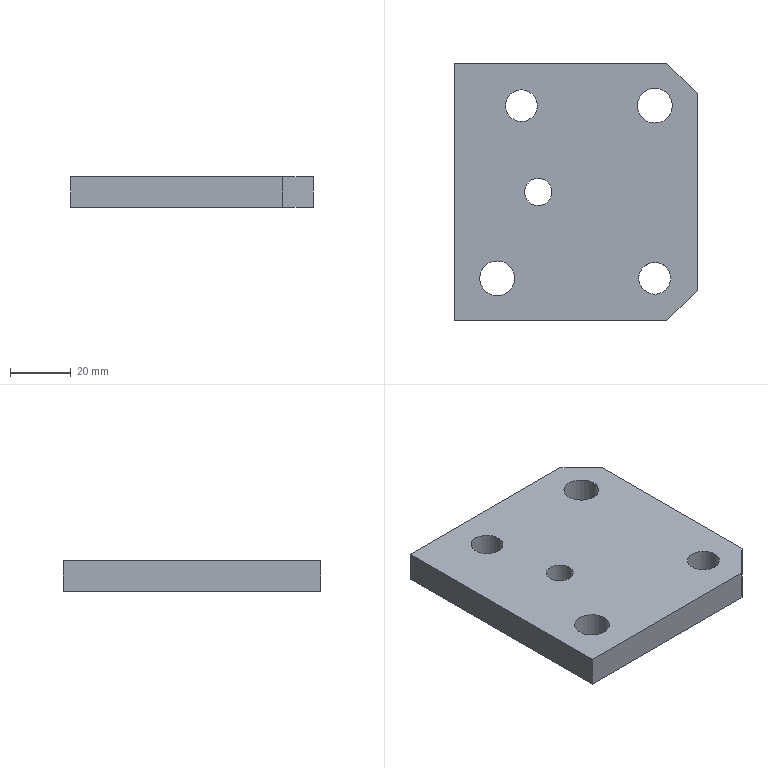Part | NX | features 6 2 | 1 solid | 13 faces | box 80 x 85 x 10 mm | volume 62555 mm3 | plane 8 | cylinder 5 | commonest cylinder face diameters 10.5 x2 11.5 x2 9 x1
STEP:
#1=CARTESIAN_POINT('',(-28.694,42.5,101.));
#2=VERTEX_POINT('',#1);
#3=CARTESIAN_POINT('',(-28.694,-42.5,101.));
#4=VERTEX_POINT('',#3);
#5=CARTESIAN_POINT('',(-28.694,0.,101.));
#6=DIRECTION('',(0.,-1.,0.));
#7=VECTOR('',#6,1000.);
#8=LINE('',#5,#7);
#9=EDGE_CURVE('',#2,#4,#8,.T.);
#10=ORIENTED_EDGE('',*,*,#9,.F.);
#11=CARTESIAN_POINT('',(-28.694,42.5,91.));
#12=VERTEX_POINT('',#11);
#13=CARTESIAN_POINT('',(-28.694,42.5,91.));
#14=DIRECTION('',(0.,0.,-1.));
#15=VECTOR('',#14,1000.);
#16=LINE('',#13,#15);
#17=EDGE_CURVE('',#2,#12,#16,.T.);
#18=ORIENTED_EDGE('',*,*,#17,.T.);
#19=CARTESIAN_POINT('',(-28.694,-42.5,91.));
#20=VERTEX_POINT('',#19);
#21=CARTESIAN_POINT('',(-28.694,0.,91.));
#22=DIRECTION('',(0.,-1.,0.));
#23=VECTOR('',#22,1000.);
#24=LINE('',#21,#23);
#25=EDGE_CURVE('',#12,#20,#24,.T.);
#26=ORIENTED_EDGE('',*,*,#25,.T.);
#27=CARTESIAN_POINT('',(-28.694,-42.5,91.));
#28=DIRECTION('',(0.,0.,1.));
#29=VECTOR('',#28,1000.);
#30=LINE('',#27,#29);
#31=EDGE_CURVE('',#20,#4,#30,.T.);
#32=ORIENTED_EDGE('',*,*,#31,.T.);
#33=EDGE_LOOP('',(#10,#18,#26,#32));
#34=FACE_BOUND('',#33,.T.);
#35=CARTESIAN_POINT('',(-28.694,0.,91.));
#36=DIRECTION('',(1.,0.,0.));
#37=DIRECTION('',(0.,-1.,0.));
#38=AXIS2_PLACEMENT_3D('',#35,#36,#37);
#39=PLANE('',#38);
#40=ADVANCED_FACE('',(#34),#39,.F.);
#41=CARTESIAN_POINT('',(41.306,42.5,101.));
#42=VERTEX_POINT('',#41);
#43=CARTESIAN_POINT('',(21.306,42.5,101.));
#44=DIRECTION('',(-1.,0.,0.));
#45=VECTOR('',#44,1000.);
#46=LINE('',#43,#45);
#47=EDGE_CURVE('',#42,#2,#46,.T.);
#48=ORIENTED_EDGE('',*,*,#47,.F.);
#49=CARTESIAN_POINT('',(41.306,42.5,91.));
#50=VERTEX_POINT('',#49);
#51=CARTESIAN_POINT('',(41.306,42.5,91.));
#52=DIRECTION('',(0.,0.,-1.));
#53=VECTOR('',#52,1000.);
#54=LINE('',#51,#53);
#55=EDGE_CURVE('',#42,#50,#54,.T.);
#56=ORIENTED_EDGE('',*,*,#55,.T.);
#57=CARTESIAN_POINT('',(21.306,42.5,91.));
#58=DIRECTION('',(-1.,0.,0.));
#59=VECTOR('',#58,1000.);
#60=LINE('',#57,#59);
#61=EDGE_CURVE('',#50,#12,#60,.T.);
#62=ORIENTED_EDGE('',*,*,#61,.T.);
#63=ORIENTED_EDGE('',*,*,#17,.F.);
#64=EDGE_LOOP('',(#48,#56,#62,#63));
#65=FACE_BOUND('',#64,.T.);
#66=CARTESIAN_POINT('',(21.306,42.5,91.));
#67=DIRECTION('',(0.,-1.,0.));
#68=DIRECTION('',(-1.,0.,0.));
#69=AXIS2_PLACEMENT_3D('',#66,#67,#68);
#70=PLANE('',#69);
#71=ADVANCED_FACE('',(#65),#70,.F.);
#72=CARTESIAN_POINT('',(51.306,-32.5,101.));
#73=VERTEX_POINT('',#72);
#74=CARTESIAN_POINT('',(51.306,32.5,101.));
#75=VERTEX_POINT('',#74);
#76=CARTESIAN_POINT('',(51.306,0.,101.));
#77=DIRECTION('',(0.,1.,0.));
#78=VECTOR('',#77,1000.);
#79=LINE('',#76,#78);
#80=EDGE_CURVE('',#73,#75,#79,.T.);
#81=ORIENTED_EDGE('',*,*,#80,.F.);
#82=CARTESIAN_POINT('',(51.306,-32.5,91.));
#83=VERTEX_POINT('',#82);
#84=CARTESIAN_POINT('',(51.306,-32.5,91.));
#85=DIRECTION('',(0.,0.,-1.));
#86=VECTOR('',#85,1000.);
#87=LINE('',#84,#86);
#88=EDGE_CURVE('',#73,#83,#87,.T.);
#89=ORIENTED_EDGE('',*,*,#88,.T.);
#90=CARTESIAN_POINT('',(51.306,32.5,91.));
#91=VERTEX_POINT('',#90);
#92=CARTESIAN_POINT('',(51.306,0.,91.));
#93=DIRECTION('',(0.,1.,0.));
#94=VECTOR('',#93,1000.);
#95=LINE('',#92,#94);
#96=EDGE_CURVE('',#83,#91,#95,.T.);
#97=ORIENTED_EDGE('',*,*,#96,.T.);
#98=CARTESIAN_POINT('',(51.306,32.5,91.));
#99=DIRECTION('',(0.,0.,1.));
#100=VECTOR('',#99,1000.);
#101=LINE('',#98,#100);
#102=EDGE_CURVE('',#91,#75,#101,.T.);
#103=ORIENTED_EDGE('',*,*,#102,.T.);
#104=EDGE_LOOP('',(#81,#89,#97,#103));
#105=FACE_BOUND('',#104,.T.);
#106=CARTESIAN_POINT('',(51.306,0.,91.));
#107=DIRECTION('',(-1.,0.,0.));
#108=DIRECTION('',(0.,1.,0.));
#109=AXIS2_PLACEMENT_3D('',#106,#107,#108);
#110=PLANE('',#109);
#111=ADVANCED_FACE('',(#105),#110,.F.);
#112=CARTESIAN_POINT('',(37.306,-33.75,91.));
#113=VERTEX_POINT('',#112);
#114=CARTESIAN_POINT('',(37.306,-28.5,91.));
#115=DIRECTION('',(0.,0.,1.));
#116=DIRECTION('',(0.,-1.,0.));
#117=AXIS2_PLACEMENT_3D('',#114,#115,#116);
#118=CIRCLE('',#117,5.25);
#119=EDGE_CURVE('',#113,#113,#118,.T.);
#120=ORIENTED_EDGE('',*,*,#119,.F.);
#121=EDGE_LOOP('',(#120));
#122=FACE_BOUND('',#121,.T.);
#123=CARTESIAN_POINT('',(37.306,-23.25,101.));
#124=VERTEX_POINT('',#123);
#125=CARTESIAN_POINT('',(37.306,-28.5,101.));
#126=DIRECTION('',(0.,0.,-1.));
#127=DIRECTION('',(0.,1.,0.));
#128=AXIS2_PLACEMENT_3D('',#125,#126,#127);
#129=CIRCLE('',#128,5.25);
#130=EDGE_CURVE('',#124,#124,#129,.T.);
#131=ORIENTED_EDGE('',*,*,#130,.F.);
#132=EDGE_LOOP('',(#131));
#133=FACE_BOUND('',#132,.T.);
#134=CARTESIAN_POINT('',(37.306,-28.5,91.));
#135=DIRECTION('',(0.,0.,1.));
#136=DIRECTION('',(0.,-1.,0.));
#137=AXIS2_PLACEMENT_3D('',#134,#135,#136);
#138=CYLINDRICAL_SURFACE('',#137,5.25);
#139=ADVANCED_FACE('',(#122,#133),#138,.F.);
#140=CARTESIAN_POINT('',(-14.694,-22.75,91.));
#141=VERTEX_POINT('',#140);
#142=CARTESIAN_POINT('',(-14.694,-28.5,91.));
#143=DIRECTION('',(0.,0.,-1.));
#144=DIRECTION('',(0.,1.,0.));
#145=AXIS2_PLACEMENT_3D('',#142,#143,#144);
#146=CIRCLE('',#145,5.75);
#147=EDGE_CURVE('',#141,#141,#146,.T.);
#148=ORIENTED_EDGE('',*,*,#147,.T.);
#149=EDGE_LOOP('',(#148));
#150=FACE_BOUND('',#149,.T.);
#151=CARTESIAN_POINT('',(-14.694,-22.75,101.));
#152=VERTEX_POINT('',#151);
#153=CARTESIAN_POINT('',(-14.694,-28.5,101.));
#154=DIRECTION('',(0.,0.,-1.));
#155=DIRECTION('',(0.,1.,0.));
#156=AXIS2_PLACEMENT_3D('',#153,#154,#155);
#157=CIRCLE('',#156,5.75);
#158=EDGE_CURVE('',#152,#152,#157,.T.);
#159=ORIENTED_EDGE('',*,*,#158,.F.);
#160=EDGE_LOOP('',(#159));
#161=FACE_BOUND('',#160,.T.);
#162=CARTESIAN_POINT('',(-14.694,-28.5,91.));
#163=DIRECTION('',(0.,0.,1.));
#164=DIRECTION('',(0.,-1.,0.));
#165=AXIS2_PLACEMENT_3D('',#162,#163,#164);
#166=CYLINDRICAL_SURFACE('',#165,5.75);
#167=ADVANCED_FACE('',(#150,#161),#166,.F.);
#168=CARTESIAN_POINT('',(41.306,-42.5,91.));
#169=VERTEX_POINT('',#168);
#170=CARTESIAN_POINT('',(21.306,-42.5,91.));
#171=DIRECTION('',(1.,0.,0.));
#172=VECTOR('',#171,1000.);
#173=LINE('',#170,#172);
#174=EDGE_CURVE('',#20,#169,#173,.T.);
#175=ORIENTED_EDGE('',*,*,#174,.T.);
#176=CARTESIAN_POINT('',(41.306,-42.5,101.));
#177=VERTEX_POINT('',#176);
#178=CARTESIAN_POINT('',(41.306,-42.5,91.));
#179=DIRECTION('',(0.,0.,1.));
#180=VECTOR('',#179,1000.);
#181=LINE('',#178,#180);
#182=EDGE_CURVE('',#169,#177,#181,.T.);
#183=ORIENTED_EDGE('',*,*,#182,.T.);
#184=CARTESIAN_POINT('',(21.306,-42.5,101.));
#185=DIRECTION('',(1.,0.,0.));
#186=VECTOR('',#185,1000.);
#187=LINE('',#184,#186);
#188=EDGE_CURVE('',#4,#177,#187,.T.);
#189=ORIENTED_EDGE('',*,*,#188,.F.);
#190=ORIENTED_EDGE('',*,*,#31,.F.);
#191=EDGE_LOOP('',(#175,#183,#189,#190));
#192=FACE_BOUND('',#191,.T.);
#193=CARTESIAN_POINT('',(21.306,-42.5,91.));
#194=DIRECTION('',(0.,1.,0.));
#195=DIRECTION('',(1.,0.,0.));
#196=AXIS2_PLACEMENT_3D('',#193,#194,#195);
#197=PLANE('',#196);
#198=ADVANCED_FACE('',(#192),#197,.F.);
#199=CARTESIAN_POINT('',(37.306,34.25,91.));
#200=VERTEX_POINT('',#199);
#201=CARTESIAN_POINT('',(37.306,28.5,91.));
#202=DIRECTION('',(0.,0.,-1.));
#203=DIRECTION('',(0.,1.,0.));
#204=AXIS2_PLACEMENT_3D('',#201,#202,#203);
#205=CIRCLE('',#204,5.75);
#206=EDGE_CURVE('',#200,#200,#205,.T.);
#207=ORIENTED_EDGE('',*,*,#206,.T.);
#208=EDGE_LOOP('',(#207));
#209=FACE_BOUND('',#208,.T.);
#210=CARTESIAN_POINT('',(37.306,34.25,101.));
#211=VERTEX_POINT('',#210);
#212=CARTESIAN_POINT('',(37.306,28.5,101.));
#213=DIRECTION('',(0.,0.,-1.));
#214=DIRECTION('',(0.,1.,0.));
#215=AXIS2_PLACEMENT_3D('',#212,#213,#214);
#216=CIRCLE('',#215,5.75);
#217=EDGE_CURVE('',#211,#211,#216,.T.);
#218=ORIENTED_EDGE('',*,*,#217,.F.);
#219=EDGE_LOOP('',(#218));
#220=FACE_BOUND('',#219,.T.);
#221=CARTESIAN_POINT('',(37.306,28.5,91.));
#222=DIRECTION('',(0.,0.,1.));
#223=DIRECTION('',(0.,-1.,0.));
#224=AXIS2_PLACEMENT_3D('',#221,#222,#223);
#225=CYLINDRICAL_SURFACE('',#224,5.75);
#226=ADVANCED_FACE('',(#209,#220),#225,.F.);
#227=CARTESIAN_POINT('',(-6.694,23.25,91.));
#228=VERTEX_POINT('',#227);
#229=CARTESIAN_POINT('',(-6.694,28.5,91.));
#230=DIRECTION('',(0.,0.,1.));
#231=DIRECTION('',(0.,-1.,0.));
#232=AXIS2_PLACEMENT_3D('',#229,#230,#231);
#233=CIRCLE('',#232,5.25);
#234=EDGE_CURVE('',#228,#228,#233,.T.);
#235=ORIENTED_EDGE('',*,*,#234,.F.);
#236=EDGE_LOOP('',(#235));
#237=FACE_BOUND('',#236,.T.);
#238=CARTESIAN_POINT('',(-6.694,33.75,101.));
#239=VERTEX_POINT('',#238);
#240=CARTESIAN_POINT('',(-6.694,28.5,101.));
#241=DIRECTION('',(0.,0.,-1.));
#242=DIRECTION('',(0.,1.,0.));
#243=AXIS2_PLACEMENT_3D('',#240,#241,#242);
#244=CIRCLE('',#243,5.25);
#245=EDGE_CURVE('',#239,#239,#244,.T.);
#246=ORIENTED_EDGE('',*,*,#245,.F.);
#247=EDGE_LOOP('',(#246));
#248=FACE_BOUND('',#247,.T.);
#249=CARTESIAN_POINT('',(-6.694,28.5,91.));
#250=DIRECTION('',(0.,0.,1.));
#251=DIRECTION('',(0.,-1.,0.));
#252=AXIS2_PLACEMENT_3D('',#249,#250,#251);
#253=CYLINDRICAL_SURFACE('',#252,5.25);
#254=ADVANCED_FACE('',(#237,#248),#253,.F.);
#255=CARTESIAN_POINT('',(-1.194,4.5,91.));
#256=VERTEX_POINT('',#255);
#257=CARTESIAN_POINT('',(-1.194,0.,91.));
#258=DIRECTION('',(0.,0.,1.));
#259=DIRECTION('',(0.,1.,0.));
#260=AXIS2_PLACEMENT_3D('',#257,#258,#259);
#261=CIRCLE('',#260,4.5);
#262=EDGE_CURVE('',#256,#256,#261,.T.);
#263=ORIENTED_EDGE('',*,*,#262,.F.);
#264=EDGE_LOOP('',(#263));
#265=FACE_BOUND('',#264,.T.);
#266=CARTESIAN_POINT('',(-1.194,4.5,101.));
#267=VERTEX_POINT('',#266);
#268=CARTESIAN_POINT('',(-1.194,0.,101.));
#269=DIRECTION('',(0.,0.,-1.));
#270=DIRECTION('',(0.,1.,0.));
#271=AXIS2_PLACEMENT_3D('',#268,#269,#270);
#272=CIRCLE('',#271,4.5);
#273=EDGE_CURVE('',#267,#267,#272,.T.);
#274=ORIENTED_EDGE('',*,*,#273,.F.);
#275=EDGE_LOOP('',(#274));
#276=FACE_BOUND('',#275,.T.);
#277=CARTESIAN_POINT('',(-1.194,0.,-119.));
#278=DIRECTION('',(0.,0.,1.));
#279=DIRECTION('',(0.,-1.,0.));
#280=AXIS2_PLACEMENT_3D('',#277,#278,#279);
#281=CYLINDRICAL_SURFACE('',#280,4.5);
#282=ADVANCED_FACE('',(#265,#276),#281,.F.);
#283=ORIENTED_EDGE('',*,*,#234,.T.);
#284=EDGE_LOOP('',(#283));
#285=FACE_BOUND('',#284,.T.);
#286=ORIENTED_EDGE('',*,*,#206,.F.);
#287=EDGE_LOOP('',(#286));
#288=FACE_BOUND('',#287,.T.);
#289=ORIENTED_EDGE('',*,*,#96,.F.);
#290=CARTESIAN_POINT('',(41.306,-42.5,91.));
#291=DIRECTION('',(-0.7071,-0.7071,0.));
#292=VECTOR('',#291,1000.);
#293=LINE('',#290,#292);
#294=EDGE_CURVE('',#83,#169,#293,.T.);
#295=ORIENTED_EDGE('',*,*,#294,.T.);
#296=ORIENTED_EDGE('',*,*,#174,.F.);
#297=ORIENTED_EDGE('',*,*,#25,.F.);
#298=ORIENTED_EDGE('',*,*,#61,.F.);
#299=CARTESIAN_POINT('',(51.306,32.5,91.));
#300=DIRECTION('',(0.7071,-0.7071,0.));
#301=VECTOR('',#300,1000.);
#302=LINE('',#299,#301);
#303=EDGE_CURVE('',#50,#91,#302,.T.);
#304=ORIENTED_EDGE('',*,*,#303,.T.);
#305=EDGE_LOOP('',(#289,#295,#296,#297,#298,#304));
#306=FACE_BOUND('',#305,.T.);
#307=ORIENTED_EDGE('',*,*,#147,.F.);
#308=EDGE_LOOP('',(#307));
#309=FACE_BOUND('',#308,.T.);
#310=ORIENTED_EDGE('',*,*,#119,.T.);
#311=EDGE_LOOP('',(#310));
#312=FACE_BOUND('',#311,.T.);
#313=ORIENTED_EDGE('',*,*,#262,.T.);
#314=EDGE_LOOP('',(#313));
#315=FACE_BOUND('',#314,.T.);
#316=CARTESIAN_POINT('',(21.306,0.,91.));
#317=DIRECTION('',(0.,0.,1.));
#318=DIRECTION('',(0.,-1.,0.));
#319=AXIS2_PLACEMENT_3D('',#316,#317,#318);
#320=PLANE('',#319);
#321=ADVANCED_FACE('',(#285,#288,#306,#309,#312,#315),#320,.F.);
#322=ORIENTED_EDGE('',*,*,#130,.T.);
#323=EDGE_LOOP('',(#322));
#324=FACE_BOUND('',#323,.T.);
#325=ORIENTED_EDGE('',*,*,#158,.T.);
#326=EDGE_LOOP('',(#325));
#327=FACE_BOUND('',#326,.T.);
#328=ORIENTED_EDGE('',*,*,#188,.T.);
#329=CARTESIAN_POINT('',(526.556,442.75,101.));
#330=DIRECTION('',(0.7071,0.7071,0.));
#331=VECTOR('',#330,1000.);
#332=LINE('',#329,#331);
#333=EDGE_CURVE('',#177,#73,#332,.T.);
#334=ORIENTED_EDGE('',*,*,#333,.T.);
#335=ORIENTED_EDGE('',*,*,#80,.T.);
#336=CARTESIAN_POINT('',(-603.444,687.25,101.));
#337=DIRECTION('',(-0.7071,0.7071,0.));
#338=VECTOR('',#337,1000.);
#339=LINE('',#336,#338);
#340=EDGE_CURVE('',#75,#42,#339,.T.);
#341=ORIENTED_EDGE('',*,*,#340,.T.);
#342=ORIENTED_EDGE('',*,*,#47,.T.);
#343=ORIENTED_EDGE('',*,*,#9,.T.);
#344=EDGE_LOOP('',(#328,#334,#335,#341,#342,#343));
#345=FACE_BOUND('',#344,.T.);
#346=ORIENTED_EDGE('',*,*,#217,.T.);
#347=EDGE_LOOP('',(#346));
#348=FACE_BOUND('',#347,.T.);
#349=ORIENTED_EDGE('',*,*,#245,.T.);
#350=EDGE_LOOP('',(#349));
#351=FACE_BOUND('',#350,.T.);
#352=ORIENTED_EDGE('',*,*,#273,.T.);
#353=EDGE_LOOP('',(#352));
#354=FACE_BOUND('',#353,.T.);
#355=CARTESIAN_POINT('',(-160.694,1130.,101.));
#356=DIRECTION('',(0.,0.,1.));
#357=DIRECTION('',(0.,1.,0.));
#358=AXIS2_PLACEMENT_3D('',#355,#356,#357);
#359=PLANE('',#358);
#360=ADVANCED_FACE('',(#324,#327,#345,#348,#351,#354),#359,.T.);
#361=ORIENTED_EDGE('',*,*,#303,.F.);
#362=ORIENTED_EDGE('',*,*,#55,.F.);
#363=ORIENTED_EDGE('',*,*,#340,.F.);
#364=ORIENTED_EDGE('',*,*,#102,.F.);
#365=EDGE_LOOP('',(#361,#362,#363,#364));
#366=FACE_BOUND('',#365,.T.);
#367=CARTESIAN_POINT('',(51.306,32.5,91.));
#368=DIRECTION('',(-0.7071,-0.7071,0.));
#369=DIRECTION('',(0.,0.,-1.));
#370=AXIS2_PLACEMENT_3D('',#367,#368,#369);
#371=PLANE('',#370);
#372=ADVANCED_FACE('',(#366),#371,.F.);
#373=ORIENTED_EDGE('',*,*,#294,.F.);
#374=ORIENTED_EDGE('',*,*,#88,.F.);
#375=ORIENTED_EDGE('',*,*,#333,.F.);
#376=ORIENTED_EDGE('',*,*,#182,.F.);
#377=EDGE_LOOP('',(#373,#374,#375,#376));
#378=FACE_BOUND('',#377,.T.);
#379=CARTESIAN_POINT('',(41.306,-42.5,91.));
#380=DIRECTION('',(-0.7071,0.7071,0.));
#381=DIRECTION('',(0.,0.,-1.));
#382=AXIS2_PLACEMENT_3D('',#379,#380,#381);
#383=PLANE('',#382);
#384=ADVANCED_FACE('',(#378),#383,.F.);
#385=CLOSED_SHELL('',(#40,#71,#111,#139,#167,#198,#226,#254,#282,#321,#360,#372,#384));
#386=MANIFOLD_SOLID_BREP('',#385);
#387=(LENGTH_UNIT()NAMED_UNIT(*)SI_UNIT(.MILLI.,.METRE.));
#388=UNCERTAINTY_MEASURE_WITH_UNIT(LENGTH_MEASURE(0.00001),#387,'','');
#389=(NAMED_UNIT(*)PLANE_ANGLE_UNIT()SI_UNIT($,.RADIAN.));
#390=(NAMED_UNIT(*)SI_UNIT($,.STERADIAN.)SOLID_ANGLE_UNIT());
#391=(GEOMETRIC_REPRESENTATION_CONTEXT(3)GLOBAL_UNCERTAINTY_ASSIGNED_CONTEXT((#388))GLOBAL_UNIT_ASSIGNED_CONTEXT((#387,#389,#390))REPRESENTATION_CONTEXT('',''));
#392=ADVANCED_BREP_SHAPE_REPRESENTATION('',(#386),#391);